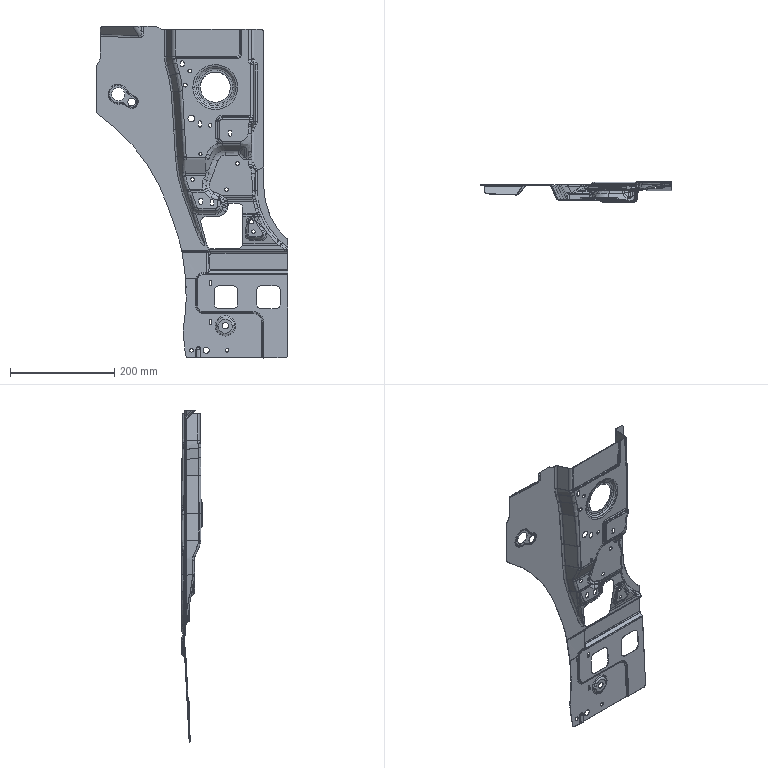Part | STEP file | FNA5401332 | 1 solid | 868 faces | box 367 x 39.355 x 636.857 mm | volume 124786 mm3 | spline 516 | cylinder 239 | plane 105 | other 6 | sphere 2 | commonest cylinder face diameters 6 x28 7 x28 12 x26 20 x16 4.4 x13 7.6 x13